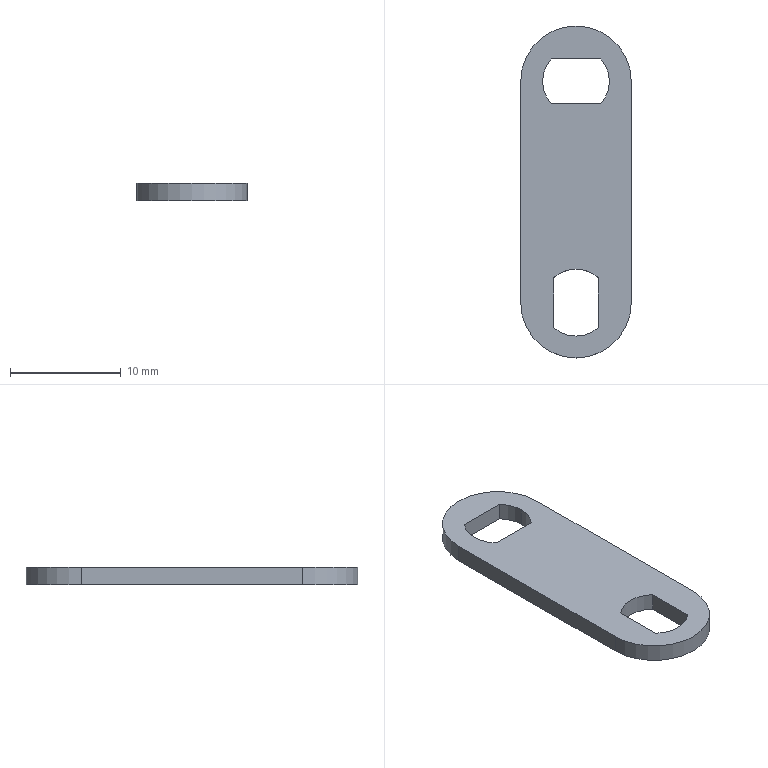Part | SolidWorks | 1 solid | 15 faces | box 10 x 30 x 1.6 mm | volume 373.587 mm3 | plane 8 | cylinder 7 | commonest cylinder face diameters 6.05 x5 10 x2
STEP:
#1=CARTESIAN_POINT('',(-2.247,17.975,-2.3));
#2=VERTEX_POINT('',#1);
#3=CARTESIAN_POINT('',(2.247,17.975,-2.3));
#4=VERTEX_POINT('',#3);
#5=CARTESIAN_POINT('',(0.,17.975,-2.3));
#6=DIRECTION('',(1.,0.,0.));
#7=VECTOR('',#6,1000.);
#8=LINE('',#5,#7);
#9=EDGE_CURVE('',#2,#4,#8,.T.);
#10=ORIENTED_EDGE('',*,*,#9,.F.);
#11=CARTESIAN_POINT('',(-2.247,17.975,-0.7));
#12=VERTEX_POINT('',#11);
#13=CARTESIAN_POINT('',(-2.247,17.975,-12.37));
#14=DIRECTION('',(0.,0.,1.));
#15=VECTOR('',#14,1000.);
#16=LINE('',#13,#15);
#17=EDGE_CURVE('',#2,#12,#16,.T.);
#18=ORIENTED_EDGE('',*,*,#17,.T.);
#19=CARTESIAN_POINT('',(2.247,17.975,-0.7));
#20=VERTEX_POINT('',#19);
#21=CARTESIAN_POINT('',(0.,17.975,-0.7));
#22=DIRECTION('',(1.,0.,0.));
#23=VECTOR('',#22,1000.);
#24=LINE('',#21,#23);
#25=EDGE_CURVE('',#12,#20,#24,.T.);
#26=ORIENTED_EDGE('',*,*,#25,.T.);
#27=CARTESIAN_POINT('',(2.247,17.975,-12.37));
#28=DIRECTION('',(0.,0.,1.));
#29=VECTOR('',#28,1000.);
#30=LINE('',#27,#29);
#31=EDGE_CURVE('',#4,#20,#30,.T.);
#32=ORIENTED_EDGE('',*,*,#31,.F.);
#33=EDGE_LOOP('',(#10,#18,#26,#32));
#34=FACE_OUTER_BOUND('',#33,.T.);
#35=CARTESIAN_POINT('',(0.,17.975,-12.37));
#36=DIRECTION('',(0.,-1.,0.));
#37=DIRECTION('',(0.,0.,-1.));
#38=AXIS2_PLACEMENT_3D('',#35,#36,#37);
#39=PLANE('',#38);
#40=ADVANCED_FACE('',(#34),#39,.F.);
#41=CARTESIAN_POINT('',(-2.247,22.025,-2.3));
#42=VERTEX_POINT('',#41);
#43=CARTESIAN_POINT('',(0.,20.,-2.3));
#44=DIRECTION('',(0.,0.,1.));
#45=DIRECTION('',(-1.,0.,0.));
#46=AXIS2_PLACEMENT_3D('',#43,#44,#45);
#47=CIRCLE('',#46,3.025);
#48=EDGE_CURVE('',#42,#2,#47,.T.);
#49=ORIENTED_EDGE('',*,*,#48,.F.);
#50=CARTESIAN_POINT('',(-2.247,22.025,-0.7));
#51=VERTEX_POINT('',#50);
#52=CARTESIAN_POINT('',(-2.247,22.025,-12.37));
#53=DIRECTION('',(0.,0.,1.));
#54=VECTOR('',#53,1000.);
#55=LINE('',#52,#54);
#56=EDGE_CURVE('',#42,#51,#55,.T.);
#57=ORIENTED_EDGE('',*,*,#56,.T.);
#58=CARTESIAN_POINT('',(0.,20.,-0.7));
#59=DIRECTION('',(0.,0.,1.));
#60=DIRECTION('',(1.,0.,0.));
#61=AXIS2_PLACEMENT_3D('',#58,#59,#60);
#62=CIRCLE('',#61,3.025);
#63=EDGE_CURVE('',#51,#12,#62,.T.);
#64=ORIENTED_EDGE('',*,*,#63,.T.);
#65=ORIENTED_EDGE('',*,*,#17,.F.);
#66=EDGE_LOOP('',(#49,#57,#64,#65));
#67=FACE_OUTER_BOUND('',#66,.T.);
#68=CARTESIAN_POINT('',(0.,20.,-12.37));
#69=DIRECTION('',(0.,0.,1.));
#70=DIRECTION('',(1.,0.,0.));
#71=AXIS2_PLACEMENT_3D('',#68,#69,#70);
#72=CYLINDRICAL_SURFACE('',#71,3.025);
#73=ADVANCED_FACE('',(#67),#72,.F.);
#74=CARTESIAN_POINT('',(2.247,22.025,-2.3));
#75=VERTEX_POINT('',#74);
#76=CARTESIAN_POINT('',(0.,22.025,-2.3));
#77=DIRECTION('',(-1.,0.,0.));
#78=VECTOR('',#77,1000.);
#79=LINE('',#76,#78);
#80=EDGE_CURVE('',#75,#42,#79,.T.);
#81=ORIENTED_EDGE('',*,*,#80,.F.);
#82=CARTESIAN_POINT('',(2.247,22.025,-0.7));
#83=VERTEX_POINT('',#82);
#84=CARTESIAN_POINT('',(2.247,22.025,-12.37));
#85=DIRECTION('',(0.,0.,1.));
#86=VECTOR('',#85,1000.);
#87=LINE('',#84,#86);
#88=EDGE_CURVE('',#75,#83,#87,.T.);
#89=ORIENTED_EDGE('',*,*,#88,.T.);
#90=CARTESIAN_POINT('',(0.,22.025,-0.7));
#91=DIRECTION('',(-1.,0.,0.));
#92=VECTOR('',#91,1000.);
#93=LINE('',#90,#92);
#94=EDGE_CURVE('',#83,#51,#93,.T.);
#95=ORIENTED_EDGE('',*,*,#94,.T.);
#96=ORIENTED_EDGE('',*,*,#56,.F.);
#97=EDGE_LOOP('',(#81,#89,#95,#96));
#98=FACE_OUTER_BOUND('',#97,.T.);
#99=CARTESIAN_POINT('',(0.,22.025,-12.37));
#100=DIRECTION('',(0.,1.,0.));
#101=DIRECTION('',(1.,0.,0.));
#102=AXIS2_PLACEMENT_3D('',#99,#100,#101);
#103=PLANE('',#102);
#104=ADVANCED_FACE('',(#98),#103,.F.);
#105=CARTESIAN_POINT('',(3.025,20.,-2.3));
#106=VERTEX_POINT('',#105);
#107=CARTESIAN_POINT('',(3.025,20.,-0.7));
#108=VERTEX_POINT('',#107);
#109=CARTESIAN_POINT('',(3.025,20.,-12.37));
#110=DIRECTION('',(0.,0.,1.));
#111=VECTOR('',#110,1000.);
#112=LINE('',#109,#111);
#113=EDGE_CURVE('',#106,#108,#112,.T.);
#114=ORIENTED_EDGE('',*,*,#113,.F.);
#115=CARTESIAN_POINT('',(0.,20.,-2.3));
#116=DIRECTION('',(0.,0.,1.));
#117=DIRECTION('',(-1.,0.,0.));
#118=AXIS2_PLACEMENT_3D('',#115,#116,#117);
#119=CIRCLE('',#118,3.025);
#120=EDGE_CURVE('',#4,#106,#119,.T.);
#121=ORIENTED_EDGE('',*,*,#120,.F.);
#122=ORIENTED_EDGE('',*,*,#31,.T.);
#123=CARTESIAN_POINT('',(0.,20.,-0.7));
#124=DIRECTION('',(0.,0.,1.));
#125=DIRECTION('',(1.,0.,0.));
#126=AXIS2_PLACEMENT_3D('',#123,#124,#125);
#127=CIRCLE('',#126,3.025);
#128=EDGE_CURVE('',#20,#108,#127,.T.);
#129=ORIENTED_EDGE('',*,*,#128,.T.);
#130=EDGE_LOOP('',(#114,#121,#122,#129));
#131=FACE_OUTER_BOUND('',#130,.T.);
#132=CARTESIAN_POINT('',(0.,20.,-12.37));
#133=DIRECTION('',(0.,0.,1.));
#134=DIRECTION('',(1.,0.,0.));
#135=AXIS2_PLACEMENT_3D('',#132,#133,#134);
#136=CYLINDRICAL_SURFACE('',#135,3.025);
#137=ADVANCED_FACE('',(#131),#136,.F.);
#138=CARTESIAN_POINT('',(2.025,-2.247,-2.3));
#139=VERTEX_POINT('',#138);
#140=CARTESIAN_POINT('',(2.025,2.247,-2.3));
#141=VERTEX_POINT('',#140);
#142=CARTESIAN_POINT('',(2.025,0.,-2.3));
#143=DIRECTION('',(0.,1.,0.));
#144=VECTOR('',#143,1000.);
#145=LINE('',#142,#144);
#146=EDGE_CURVE('',#139,#141,#145,.T.);
#147=ORIENTED_EDGE('',*,*,#146,.F.);
#148=CARTESIAN_POINT('',(2.025,-2.247,-0.7));
#149=VERTEX_POINT('',#148);
#150=CARTESIAN_POINT('',(2.025,-2.247,-12.37));
#151=DIRECTION('',(0.,0.,1.));
#152=VECTOR('',#151,1000.);
#153=LINE('',#150,#152);
#154=EDGE_CURVE('',#139,#149,#153,.T.);
#155=ORIENTED_EDGE('',*,*,#154,.T.);
#156=CARTESIAN_POINT('',(2.025,2.247,-0.7));
#157=VERTEX_POINT('',#156);
#158=CARTESIAN_POINT('',(2.025,0.,-0.7));
#159=DIRECTION('',(0.,1.,0.));
#160=VECTOR('',#159,1000.);
#161=LINE('',#158,#160);
#162=EDGE_CURVE('',#149,#157,#161,.T.);
#163=ORIENTED_EDGE('',*,*,#162,.T.);
#164=CARTESIAN_POINT('',(2.025,2.247,-12.37));
#165=DIRECTION('',(0.,0.,1.));
#166=VECTOR('',#165,1000.);
#167=LINE('',#164,#166);
#168=EDGE_CURVE('',#141,#157,#167,.T.);
#169=ORIENTED_EDGE('',*,*,#168,.F.);
#170=EDGE_LOOP('',(#147,#155,#163,#169));
#171=FACE_OUTER_BOUND('',#170,.T.);
#172=CARTESIAN_POINT('',(2.025,0.,-12.37));
#173=DIRECTION('',(1.,0.,0.));
#174=DIRECTION('',(0.,1.,0.));
#175=AXIS2_PLACEMENT_3D('',#172,#173,#174);
#176=PLANE('',#175);
#177=ADVANCED_FACE('',(#171),#176,.F.);
#178=CARTESIAN_POINT('',(-2.025,-2.247,-2.3));
#179=VERTEX_POINT('',#178);
#180=CARTESIAN_POINT('',(0.,0.,-2.3));
#181=DIRECTION('',(0.,0.,1.));
#182=DIRECTION('',(-1.,0.,0.));
#183=AXIS2_PLACEMENT_3D('',#180,#181,#182);
#184=CIRCLE('',#183,3.025);
#185=EDGE_CURVE('',#179,#139,#184,.T.);
#186=ORIENTED_EDGE('',*,*,#185,.F.);
#187=CARTESIAN_POINT('',(-2.025,-2.247,-0.7));
#188=VERTEX_POINT('',#187);
#189=CARTESIAN_POINT('',(-2.025,-2.247,-12.37));
#190=DIRECTION('',(0.,0.,1.));
#191=VECTOR('',#190,1000.);
#192=LINE('',#189,#191);
#193=EDGE_CURVE('',#179,#188,#192,.T.);
#194=ORIENTED_EDGE('',*,*,#193,.T.);
#195=CARTESIAN_POINT('',(0.,0.,-0.7));
#196=DIRECTION('',(0.,0.,1.));
#197=DIRECTION('',(1.,0.,0.));
#198=AXIS2_PLACEMENT_3D('',#195,#196,#197);
#199=CIRCLE('',#198,3.025);
#200=EDGE_CURVE('',#188,#149,#199,.T.);
#201=ORIENTED_EDGE('',*,*,#200,.T.);
#202=ORIENTED_EDGE('',*,*,#154,.F.);
#203=EDGE_LOOP('',(#186,#194,#201,#202));
#204=FACE_OUTER_BOUND('',#203,.T.);
#205=CARTESIAN_POINT('',(0.,0.,-12.37));
#206=DIRECTION('',(0.,0.,1.));
#207=DIRECTION('',(1.,0.,0.));
#208=AXIS2_PLACEMENT_3D('',#205,#206,#207);
#209=CYLINDRICAL_SURFACE('',#208,3.025);
#210=ADVANCED_FACE('',(#204),#209,.F.);
#211=CARTESIAN_POINT('',(-2.025,2.247,-2.3));
#212=VERTEX_POINT('',#211);
#213=CARTESIAN_POINT('',(-2.025,0.,-2.3));
#214=DIRECTION('',(0.,-1.,0.));
#215=VECTOR('',#214,1000.);
#216=LINE('',#213,#215);
#217=EDGE_CURVE('',#212,#179,#216,.T.);
#218=ORIENTED_EDGE('',*,*,#217,.F.);
#219=CARTESIAN_POINT('',(-2.025,2.247,-0.7));
#220=VERTEX_POINT('',#219);
#221=CARTESIAN_POINT('',(-2.025,2.247,-12.37));
#222=DIRECTION('',(0.,0.,1.));
#223=VECTOR('',#222,1000.);
#224=LINE('',#221,#223);
#225=EDGE_CURVE('',#212,#220,#224,.T.);
#226=ORIENTED_EDGE('',*,*,#225,.T.);
#227=CARTESIAN_POINT('',(-2.025,0.,-0.7));
#228=DIRECTION('',(0.,-1.,0.));
#229=VECTOR('',#228,1000.);
#230=LINE('',#227,#229);
#231=EDGE_CURVE('',#220,#188,#230,.T.);
#232=ORIENTED_EDGE('',*,*,#231,.T.);
#233=ORIENTED_EDGE('',*,*,#193,.F.);
#234=EDGE_LOOP('',(#218,#226,#232,#233));
#235=FACE_OUTER_BOUND('',#234,.T.);
#236=CARTESIAN_POINT('',(-2.025,0.,-12.37));
#237=DIRECTION('',(-1.,0.,0.));
#238=DIRECTION('',(0.,1.,0.));
#239=AXIS2_PLACEMENT_3D('',#236,#237,#238);
#240=PLANE('',#239);
#241=ADVANCED_FACE('',(#235),#240,.F.);
#242=CARTESIAN_POINT('',(0.,0.,-2.3));
#243=DIRECTION('',(0.,0.,1.));
#244=DIRECTION('',(-1.,0.,0.));
#245=AXIS2_PLACEMENT_3D('',#242,#243,#244);
#246=CIRCLE('',#245,3.025);
#247=EDGE_CURVE('',#141,#212,#246,.T.);
#248=ORIENTED_EDGE('',*,*,#247,.F.);
#249=ORIENTED_EDGE('',*,*,#168,.T.);
#250=CARTESIAN_POINT('',(0.,0.,-0.7));
#251=DIRECTION('',(0.,0.,1.));
#252=DIRECTION('',(1.,0.,0.));
#253=AXIS2_PLACEMENT_3D('',#250,#251,#252);
#254=CIRCLE('',#253,3.025);
#255=EDGE_CURVE('',#157,#220,#254,.T.);
#256=ORIENTED_EDGE('',*,*,#255,.T.);
#257=ORIENTED_EDGE('',*,*,#225,.F.);
#258=EDGE_LOOP('',(#248,#249,#256,#257));
#259=FACE_OUTER_BOUND('',#258,.T.);
#260=CARTESIAN_POINT('',(0.,0.,-12.37));
#261=DIRECTION('',(0.,0.,1.));
#262=DIRECTION('',(1.,0.,0.));
#263=AXIS2_PLACEMENT_3D('',#260,#261,#262);
#264=CYLINDRICAL_SURFACE('',#263,3.025);
#265=ADVANCED_FACE('',(#259),#264,.F.);
#266=CARTESIAN_POINT('',(5.,0.,-0.7));
#267=VERTEX_POINT('',#266);
#268=CARTESIAN_POINT('',(5.,20.,-0.7));
#269=VERTEX_POINT('',#268);
#270=CARTESIAN_POINT('',(5.,0.,-0.7));
#271=DIRECTION('',(0.,1.,0.));
#272=VECTOR('',#271,1000.);
#273=LINE('',#270,#272);
#274=EDGE_CURVE('',#267,#269,#273,.T.);
#275=ORIENTED_EDGE('',*,*,#274,.F.);
#276=CARTESIAN_POINT('',(5.,0.,-2.3));
#277=VERTEX_POINT('',#276);
#278=CARTESIAN_POINT('',(5.,0.,-2.3));
#279=DIRECTION('',(0.,0.,1.));
#280=VECTOR('',#279,1000.);
#281=LINE('',#278,#280);
#282=EDGE_CURVE('',#277,#267,#281,.T.);
#283=ORIENTED_EDGE('',*,*,#282,.F.);
#284=CARTESIAN_POINT('',(5.,20.,-2.3));
#285=VERTEX_POINT('',#284);
#286=CARTESIAN_POINT('',(5.,0.,-2.3));
#287=DIRECTION('',(0.,1.,0.));
#288=VECTOR('',#287,1000.);
#289=LINE('',#286,#288);
#290=EDGE_CURVE('',#277,#285,#289,.T.);
#291=ORIENTED_EDGE('',*,*,#290,.T.);
#292=CARTESIAN_POINT('',(5.,20.,-2.3));
#293=DIRECTION('',(0.,0.,1.));
#294=VECTOR('',#293,1000.);
#295=LINE('',#292,#294);
#296=EDGE_CURVE('',#285,#269,#295,.T.);
#297=ORIENTED_EDGE('',*,*,#296,.T.);
#298=EDGE_LOOP('',(#275,#283,#291,#297));
#299=FACE_OUTER_BOUND('',#298,.T.);
#300=CARTESIAN_POINT('',(5.,0.,-2.3));
#301=DIRECTION('',(1.,0.,0.));
#302=DIRECTION('',(0.,1.,0.));
#303=AXIS2_PLACEMENT_3D('',#300,#301,#302);
#304=PLANE('',#303);
#305=ADVANCED_FACE('',(#299),#304,.T.);
#306=CARTESIAN_POINT('',(-5.,20.,-0.7));
#307=VERTEX_POINT('',#306);
#308=CARTESIAN_POINT('',(0.,20.,-0.7));
#309=DIRECTION('',(0.,0.,1.));
#310=DIRECTION('',(1.,0.,0.));
#311=AXIS2_PLACEMENT_3D('',#308,#309,#310);
#312=CIRCLE('',#311,5.);
#313=EDGE_CURVE('',#269,#307,#312,.T.);
#314=ORIENTED_EDGE('',*,*,#313,.F.);
#315=ORIENTED_EDGE('',*,*,#296,.F.);
#316=CARTESIAN_POINT('',(-5.,20.,-2.3));
#317=VERTEX_POINT('',#316);
#318=CARTESIAN_POINT('',(0.,20.,-2.3));
#319=DIRECTION('',(0.,0.,1.));
#320=DIRECTION('',(1.,0.,0.));
#321=AXIS2_PLACEMENT_3D('',#318,#319,#320);
#322=CIRCLE('',#321,5.);
#323=EDGE_CURVE('',#285,#317,#322,.T.);
#324=ORIENTED_EDGE('',*,*,#323,.T.);
#325=CARTESIAN_POINT('',(-5.,20.,-2.3));
#326=DIRECTION('',(0.,0.,1.));
#327=VECTOR('',#326,1000.);
#328=LINE('',#325,#327);
#329=EDGE_CURVE('',#317,#307,#328,.T.);
#330=ORIENTED_EDGE('',*,*,#329,.T.);
#331=EDGE_LOOP('',(#314,#315,#324,#330));
#332=FACE_OUTER_BOUND('',#331,.T.);
#333=CARTESIAN_POINT('',(0.,20.,-2.3));
#334=DIRECTION('',(0.,0.,1.));
#335=DIRECTION('',(1.,0.,0.));
#336=AXIS2_PLACEMENT_3D('',#333,#334,#335);
#337=CYLINDRICAL_SURFACE('',#336,5.);
#338=ADVANCED_FACE('',(#332),#337,.T.);
#339=CARTESIAN_POINT('',(-5.,0.,-0.7));
#340=VERTEX_POINT('',#339);
#341=CARTESIAN_POINT('',(-5.,20.,-0.7));
#342=DIRECTION('',(0.,-1.,0.));
#343=VECTOR('',#342,1000.);
#344=LINE('',#341,#343);
#345=EDGE_CURVE('',#307,#340,#344,.T.);
#346=ORIENTED_EDGE('',*,*,#345,.F.);
#347=ORIENTED_EDGE('',*,*,#329,.F.);
#348=CARTESIAN_POINT('',(-5.,0.,-2.3));
#349=VERTEX_POINT('',#348);
#350=CARTESIAN_POINT('',(-5.,20.,-2.3));
#351=DIRECTION('',(0.,-1.,0.));
#352=VECTOR('',#351,1000.);
#353=LINE('',#350,#352);
#354=EDGE_CURVE('',#317,#349,#353,.T.);
#355=ORIENTED_EDGE('',*,*,#354,.T.);
#356=CARTESIAN_POINT('',(-5.,0.,-2.3));
#357=DIRECTION('',(0.,0.,1.));
#358=VECTOR('',#357,1000.);
#359=LINE('',#356,#358);
#360=EDGE_CURVE('',#349,#340,#359,.T.);
#361=ORIENTED_EDGE('',*,*,#360,.T.);
#362=EDGE_LOOP('',(#346,#347,#355,#361));
#363=FACE_OUTER_BOUND('',#362,.T.);
#364=CARTESIAN_POINT('',(-5.,20.,-2.3));
#365=DIRECTION('',(-1.,0.,0.));
#366=DIRECTION('',(0.,0.,1.));
#367=AXIS2_PLACEMENT_3D('',#364,#365,#366);
#368=PLANE('',#367);
#369=ADVANCED_FACE('',(#363),#368,.T.);
#370=CARTESIAN_POINT('',(0.,0.,-0.7));
#371=DIRECTION('',(0.,0.,1.));
#372=DIRECTION('',(1.,0.,0.));
#373=AXIS2_PLACEMENT_3D('',#370,#371,#372);
#374=CIRCLE('',#373,5.);
#375=EDGE_CURVE('',#340,#267,#374,.T.);
#376=ORIENTED_EDGE('',*,*,#375,.F.);
#377=ORIENTED_EDGE('',*,*,#360,.F.);
#378=CARTESIAN_POINT('',(0.,0.,-2.3));
#379=DIRECTION('',(0.,0.,1.));
#380=DIRECTION('',(1.,0.,0.));
#381=AXIS2_PLACEMENT_3D('',#378,#379,#380);
#382=CIRCLE('',#381,5.);
#383=EDGE_CURVE('',#349,#277,#382,.T.);
#384=ORIENTED_EDGE('',*,*,#383,.T.);
#385=ORIENTED_EDGE('',*,*,#282,.T.);
#386=EDGE_LOOP('',(#376,#377,#384,#385));
#387=FACE_OUTER_BOUND('',#386,.T.);
#388=CARTESIAN_POINT('',(0.,0.,-2.3));
#389=DIRECTION('',(0.,0.,1.));
#390=DIRECTION('',(1.,0.,0.));
#391=AXIS2_PLACEMENT_3D('',#388,#389,#390);
#392=CYLINDRICAL_SURFACE('',#391,5.);
#393=ADVANCED_FACE('',(#387),#392,.T.);
#394=ORIENTED_EDGE('',*,*,#128,.F.);
#395=ORIENTED_EDGE('',*,*,#25,.F.);
#396=ORIENTED_EDGE('',*,*,#63,.F.);
#397=ORIENTED_EDGE('',*,*,#94,.F.);
#398=CARTESIAN_POINT('',(0.,20.,-0.7));
#399=DIRECTION('',(0.,0.,1.));
#400=DIRECTION('',(1.,0.,0.));
#401=AXIS2_PLACEMENT_3D('',#398,#399,#400);
#402=CIRCLE('',#401,3.025);
#403=EDGE_CURVE('',#108,#83,#402,.T.);
#404=ORIENTED_EDGE('',*,*,#403,.F.);
#405=EDGE_LOOP('',(#394,#395,#396,#397,#404));
#406=FACE_BOUND('',#405,.T.);
#407=ORIENTED_EDGE('',*,*,#255,.F.);
#408=ORIENTED_EDGE('',*,*,#162,.F.);
#409=ORIENTED_EDGE('',*,*,#200,.F.);
#410=ORIENTED_EDGE('',*,*,#231,.F.);
#411=EDGE_LOOP('',(#407,#408,#409,#410));
#412=FACE_BOUND('',#411,.T.);
#413=ORIENTED_EDGE('',*,*,#375,.T.);
#414=ORIENTED_EDGE('',*,*,#274,.T.);
#415=ORIENTED_EDGE('',*,*,#313,.T.);
#416=ORIENTED_EDGE('',*,*,#345,.T.);
#417=EDGE_LOOP('',(#413,#414,#415,#416));
#418=FACE_OUTER_BOUND('',#417,.T.);
#419=CARTESIAN_POINT('',(0.,-6.,-0.7));
#420=DIRECTION('',(0.,0.,-1.));
#421=DIRECTION('',(0.,-1.,0.));
#422=AXIS2_PLACEMENT_3D('',#419,#420,#421);
#423=PLANE('',#422);
#424=ADVANCED_FACE('',(#406,#412,#418),#423,.F.);
#425=ORIENTED_EDGE('',*,*,#9,.T.);
#426=ORIENTED_EDGE('',*,*,#120,.T.);
#427=CARTESIAN_POINT('',(0.,20.,-2.3));
#428=DIRECTION('',(0.,0.,1.));
#429=DIRECTION('',(-1.,0.,0.));
#430=AXIS2_PLACEMENT_3D('',#427,#428,#429);
#431=CIRCLE('',#430,3.025);
#432=EDGE_CURVE('',#106,#75,#431,.T.);
#433=ORIENTED_EDGE('',*,*,#432,.T.);
#434=ORIENTED_EDGE('',*,*,#80,.T.);
#435=ORIENTED_EDGE('',*,*,#48,.T.);
#436=EDGE_LOOP('',(#425,#426,#433,#434,#435));
#437=FACE_BOUND('',#436,.T.);
#438=ORIENTED_EDGE('',*,*,#146,.T.);
#439=ORIENTED_EDGE('',*,*,#247,.T.);
#440=ORIENTED_EDGE('',*,*,#217,.T.);
#441=ORIENTED_EDGE('',*,*,#185,.T.);
#442=EDGE_LOOP('',(#438,#439,#440,#441));
#443=FACE_BOUND('',#442,.T.);
#444=ORIENTED_EDGE('',*,*,#290,.F.);
#445=ORIENTED_EDGE('',*,*,#383,.F.);
#446=ORIENTED_EDGE('',*,*,#354,.F.);
#447=ORIENTED_EDGE('',*,*,#323,.F.);
#448=EDGE_LOOP('',(#444,#445,#446,#447));
#449=FACE_OUTER_BOUND('',#448,.T.);
#450=CARTESIAN_POINT('',(0.,0.,-2.3));
#451=DIRECTION('',(0.,0.,-1.));
#452=DIRECTION('',(0.,-1.,0.));
#453=AXIS2_PLACEMENT_3D('',#450,#451,#452);
#454=PLANE('',#453);
#455=ADVANCED_FACE('',(#437,#443,#449),#454,.T.);
#456=ORIENTED_EDGE('',*,*,#432,.F.);
#457=ORIENTED_EDGE('',*,*,#113,.T.);
#458=ORIENTED_EDGE('',*,*,#403,.T.);
#459=ORIENTED_EDGE('',*,*,#88,.F.);
#460=EDGE_LOOP('',(#456,#457,#458,#459));
#461=FACE_OUTER_BOUND('',#460,.T.);
#462=CARTESIAN_POINT('',(0.,20.,-12.37));
#463=DIRECTION('',(0.,0.,1.));
#464=DIRECTION('',(1.,0.,0.));
#465=AXIS2_PLACEMENT_3D('',#462,#463,#464);
#466=CYLINDRICAL_SURFACE('',#465,3.025);
#467=ADVANCED_FACE('',(#461),#466,.F.);
#468=CLOSED_SHELL('',(#40,#73,#104,#137,#177,#210,#241,#265,#305,#338,#369,#393,#424,#455,#467));
#469=MANIFOLD_SOLID_BREP('',#468);
#470=CARTESIAN_POINT('',(0.,0.,0.));
#471=DIRECTION('',(0.,0.,1.));
#472=DIRECTION('',(1.,0.,0.));
#473=AXIS2_PLACEMENT_3D('',#470,#471,#472);
#474=(LENGTH_UNIT()NAMED_UNIT(*)SI_UNIT(.MILLI.,.METRE.));
#475=UNCERTAINTY_MEASURE_WITH_UNIT(LENGTH_MEASURE(0.00001),#474,'','');
#476=(NAMED_UNIT(*)PLANE_ANGLE_UNIT()SI_UNIT($,.RADIAN.));
#477=(NAMED_UNIT(*)SI_UNIT($,.STERADIAN.)SOLID_ANGLE_UNIT());
#478=(GEOMETRIC_REPRESENTATION_CONTEXT(3)GLOBAL_UNCERTAINTY_ASSIGNED_CONTEXT((#475))GLOBAL_UNIT_ASSIGNED_CONTEXT((#474,#476,#477))REPRESENTATION_CONTEXT('',''));
#479=ADVANCED_BREP_SHAPE_REPRESENTATION('',(#469,#473),#478);